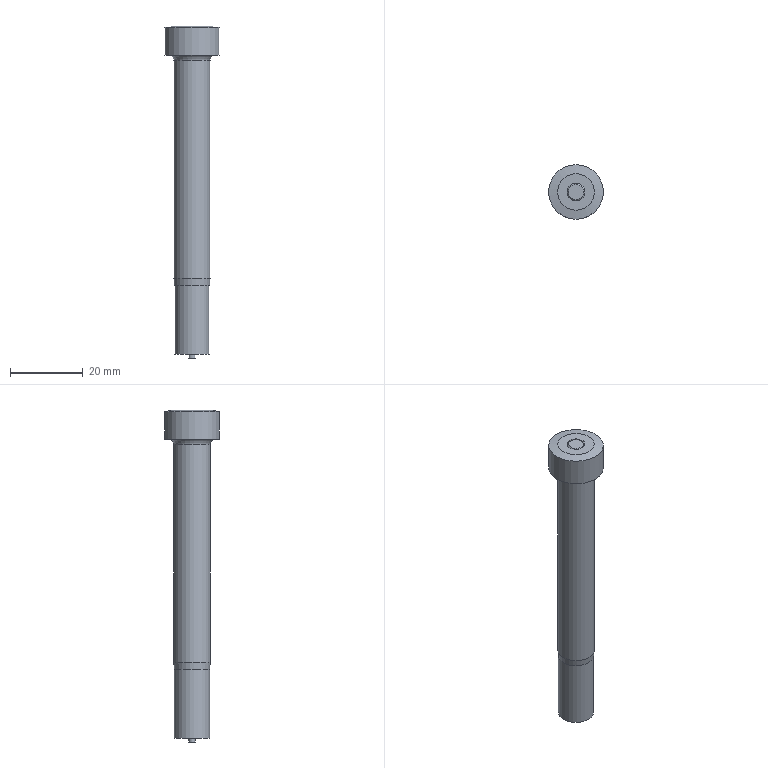Part | STEP file | 1_id2898_x_t | 1 solid | 22 faces | box 15 x 15 x 91 mm | volume 7738 mm3 | cylinder 9 | plane 8 | cone 2 | torus 2 | spline 1 | commonest cylinder face diameters 1.8 x2 4.4 x1 4.401 x1 4.9 x1 4.901 x1 9.65 x1